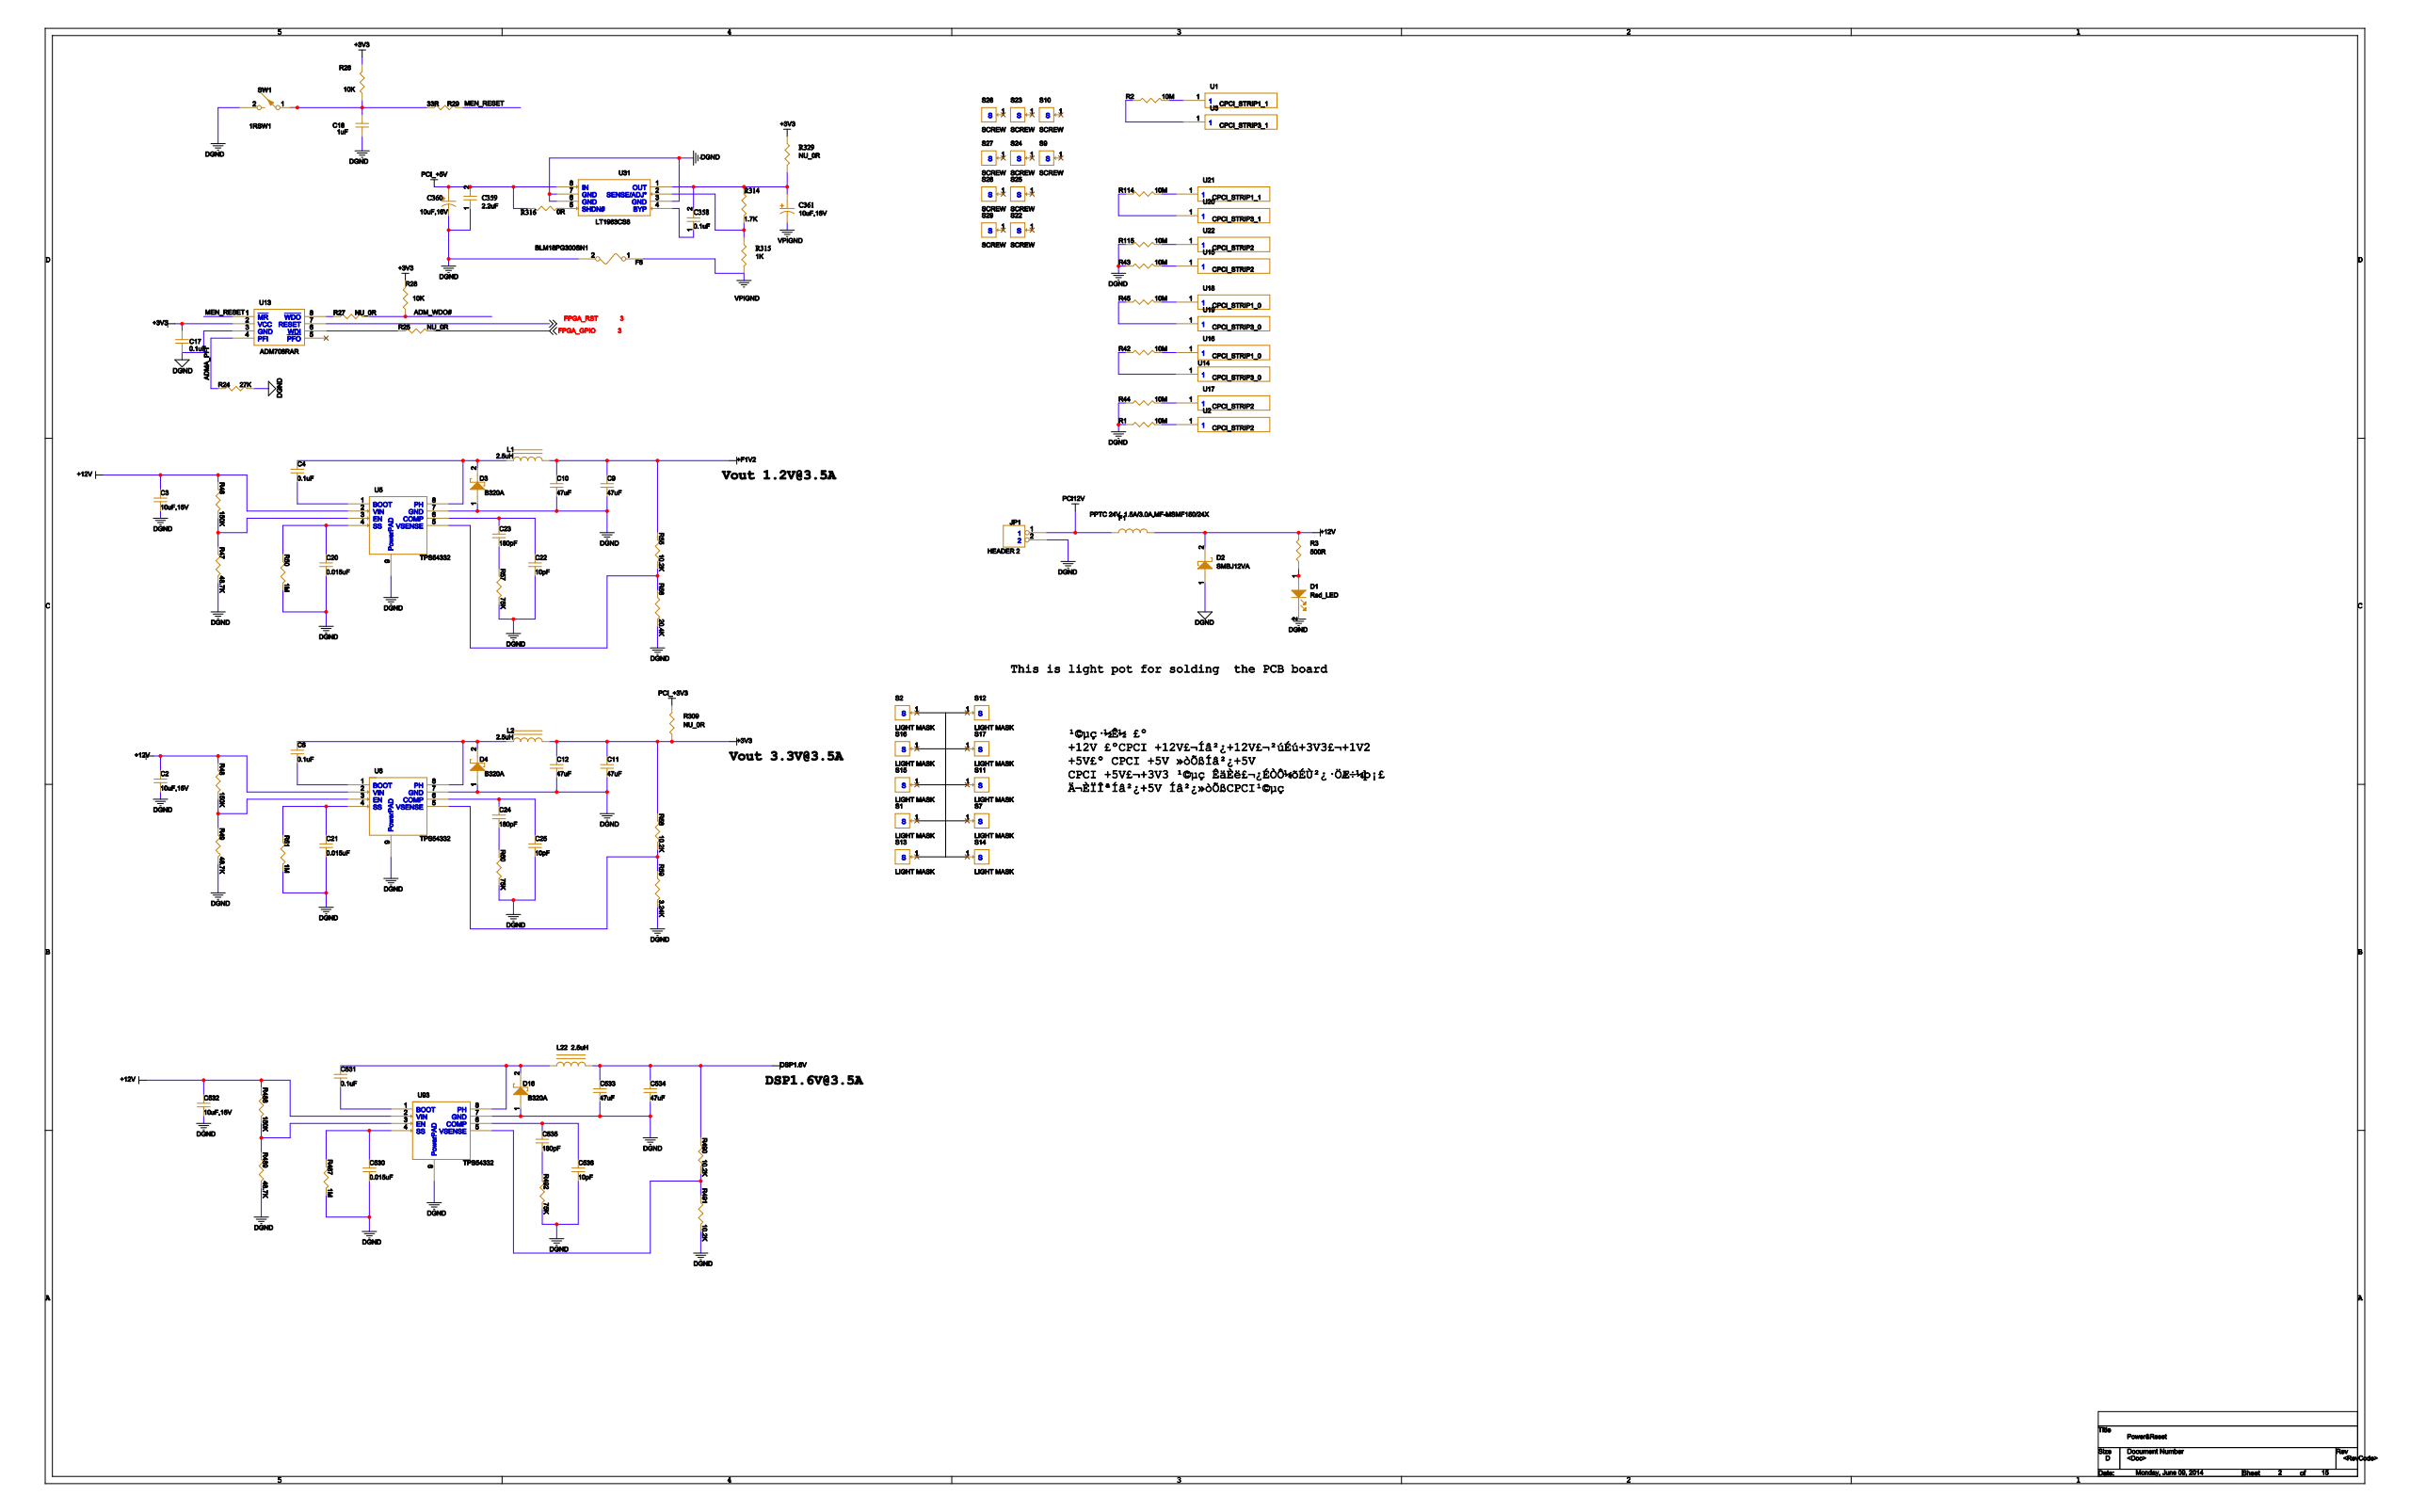Circuit board | Cadence Allegro | 669 parts | 806 nets | one sheet of the schematic
Parts on this sheet (reference | value | footprint):
C9 | 47uF | CP3528
C10 | 47uF | CP3528
C11 | 47uF | CP3528
C12 | 47uF | CP3528
C17 | 0.1uF | C0402
C20 | 0.015uF | C0402
C21 | 0.015uF | C0402
C22 | 10pF | C0402
C23 | 180pF | C0402
C24 | 180pF | C0402
C25 | 10pF | C0402
C358 | 0.1uF | C0402
C359 | 2.2uF | C0603
C361 | 10uF,16V | CP3216
C530 | 0.015uF | C0402
C531 | 0.1uF | C0402
C532 | 10uF,16V | CP3216
C533 | 47uF | CP3528
C534 | 47uF | CP3528
C535 | 180pF | C0402
C536 | 10pF | C0402
D2 | SMBJ12VA | DO214AA
D3 | B320A | B320A
D4 | B320A | B320A
D16 | B320A | B320A
F6 | BLM18PG300SN1 | F0603
JP1 | HEADER 2 | POWER_2_B
L1 | 2.5uH | MSS1038
L2 | 2.5uH | MSS1038
L22 | 2.5uH | MSS1038
R1 | 10M | R0603
R2 | 10M | R0603
R3 | 500R | R0603
R24 | 27K | R0603
R25 | NU_0R | R0603
R26 | 10K | R0603
R27 | NU_0R | R0603
R28 | 10K | R0603
R29 | 33R | R0603
R42 | 10M | R0603
R43 | 10M | R0603
R44 | 10M | R0603
R45 | 10M | R0603
R46 | 150K | R0603
R47 | 48.7K | R0603
R48 | 150K | R0603
R49 | 48.7K | R0603
R50 | 1M | R0603
R51 | 1M | R0603
R55 | 10.2K | R0603
R56 | 20.4K | R0603
R57 | 75K | R0603
R58 | 10.2K | R0603
R59 | 3.24K | R0603
R60 | 75K | R0603
R114 | 10M | R0603
R115 | 10M | R0603
R309 | NU_0R | R1210
R314 | 1.7K | R0603
R315 | 1K | R0603
R316 | 0R | R0603
R329 | NU_0R | R0603
R487 | 1M | R0603
R488 | 150K | R0603
R489 | 48.7K | R0603
R490 | 10.2K | R0603
R491 | 10.2K | R0603
R492 | 75K | R0603
SW1 | 1RSW1 | SW_2PIN
U1 | CPCI_STRIP1_1 | CPCI_STRIP1_1
U2 | CPCI_STRIP2 | CPCI_STRIP2
U3 | CPCI_STRIP3_1 | CPCI_STRIP3_1
U5 | TPS54332 | HSO8
U6 | TPS54332 | HSO8
U13 | ADM706RAR | SOP8-50-150
U14 | CPCI_STRIP3_0 | CPCI_STRIP3_0
U15 | CPCI_STRIP2 | CPCI_STRIP2
U16 | CPCI_STRIP1_0 | CPCI_STRIP1_0
U17 | CPCI_STRIP2 | CPCI_STRIP2
U18 | CPCI_STRIP1_0 | CPCI_STRIP1_0
U19 | CPCI_STRIP3_0 | CPCI_STRIP3_0
U20 | CPCI_STRIP3_1 | CPCI_STRIP3_1
U21 | CPCI_STRIP1_1 | CPCI_STRIP1_1
U22 | CPCI_STRIP2 | CPCI_STRIP2
U31 | LT1963CS8 | SO8
U93 | TPS54332 | HSO8
Nets of these parts (net: part-pin ...):
DGND: C9-2 C10-2 C11-2 C12-2 C17-2 C20-2 C21-2 C22-2 C25-2 C359-1 C530-2 C532-2 C533-2 C534-2 C536-2 D2-1 D3-1 D4-1 D16-1 F6-2 JP1-2 R1-1 R24-2 R43-1 R44-1 R47-2 R49-2 R50-2 R51-2 R56-2 R57-2 R59-2 R60-2 R115-1 R487-2 R489-2 R491-2 R492-2 SW1-2 U5-7 U5-9 U6-7 U6-9 U13-3 U31-3 U31-6 U31-7 U93-7 U93-9
+F1V2: C9-1 C10-1 L1-1 R55-1
+3V3: C11-1 C12-1 C17-1 L2-1 R26-1 R28-2 R58-1 R309-1 R329-1 U13-2
FPGA_GPIO: R25-2
FPGA_RST: U13-7
PCI_+3V3: R309-2
N17037228: R25-1 U13-6
N50997074: R27-1 U13-8
ADM_WDO#: R27-2 R28-1
N60910308: C358-2 C361-1 R314-1 R329-2 U31-1
PCI_+5V: C359-2 R316-2 U31-8
VPIGND: C361-2 F6-1 R315-2
+12V: C532-1 D2-2 R3-2 R46-1 R48-1 R488-1 U5-2 U6-2 U93-2
N61174592: C530-1 R487-1 U93-4
N53686258: C20-1 R50-1 U5-4
N53728803: C21-1 R51-1 U6-4
N61174488: C535-1 C536-1 U93-6
N53661797: C22-1 C23-1 U5-6
N53728646: C24-1 C25-1 U6-6
N61174700: C535-2 R492-1
N53663464: C23-2 R57-1
N53728907: C24-2 R60-1
N57531731: R1-2 U2-1
N57531603: R114-1 U20-1
N57531573: R114-2 U21-1
N57531633: R115-2 U22-1
N57531585: R2-1 U3-1
N57531571: R2-2 U1-1
N57531699: R42-1 U14-1
N57531735: R42-2 U16-1
N57531635: R43-2 U15-1
N57531729: R44-2 U17-1
N57531601: R45-1 U19-1
N57531745: R45-2 U18-1
MEN_RESET: R29-1 U13-1
N17039343: R26-2 R29-2 SW1-1
N61560600: R316-1 U31-5
N55364546: R3-1
PCI12V: JP1-1
N60910292: R314-2 R315-1 U31-2
DSP1.6V: C533-1 C534-1 L22-1 R490-1
N61174482: C531-1 D16-2 L22-2 U93-8
N53629509: D3-2 L1-2 U5-8
N53728644: D4-2 L2-2 U6-8
N60910318: C358-1 U31-4
N61174426: R490-2 R491-1 U93-5
N53653226: R55-2 R56-1 U5-5
N53728588: R58-2 R59-1 U6-5
N61174450: R488-2 R489-1 U93-3
N53700966: R46-2 R47-1 U5-3
N53728608: R48-2 R49-1 U6-3
N61174434: C531-2 U93-1
N53627874: U5-1
N53728592: U6-1
ADMA_PFI: R24-1 U13-4